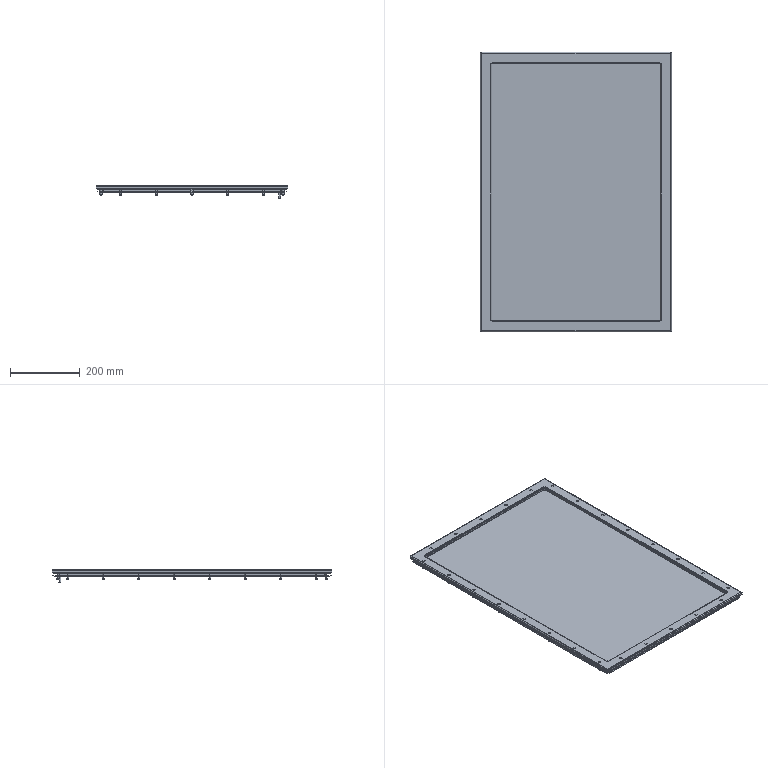Part | SolidWorks | features BaseBody 4 | 4 solids | 387 faces | box 546.1 x 800.1 x 36.322 mm | volume 3357430 mm3 | cylinder 194 | plane 139 | cone 54 | commonest cylinder face diameters 7.95 x104 6 x52 2.54 x8 3.048 x8 6.553 x8 25.4 x8